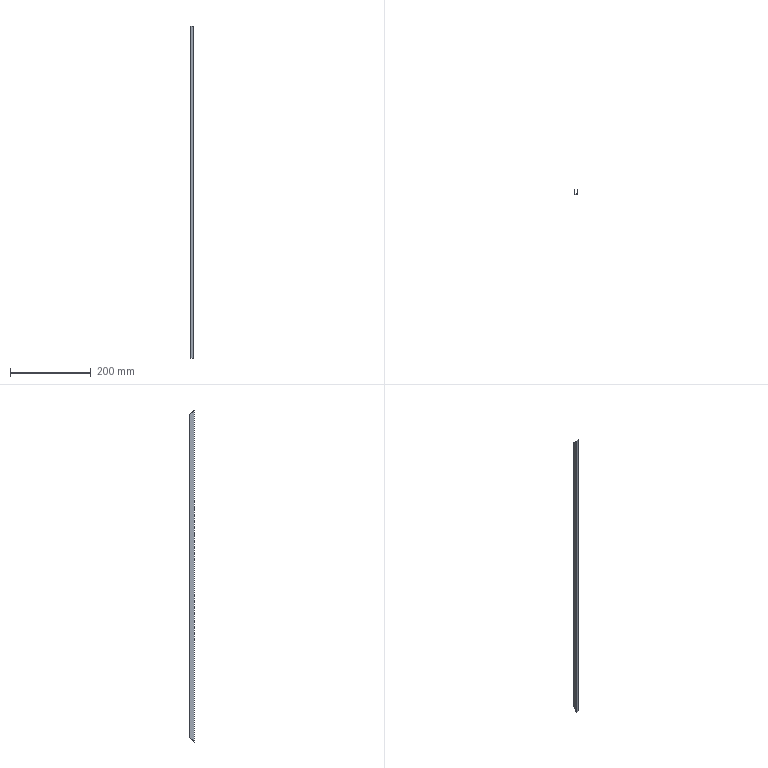Part | STEP file | Friction strip L824 | 1 solid | 10 faces | box 7 x 11 x 824 mm | volume 22001 mm3 | plane 10
STEP:
#1=CARTESIAN_POINT('',(0.,0.,0.));
#2=DIRECTION('',(0.,0.,1.));
#3=DIRECTION('',(1.,0.,0.));
#4=AXIS2_PLACEMENT_3D('',#1,#2,#3);
#5=CARTESIAN_POINT('',(3.5,0.,824.));
#6=VERTEX_POINT('',#5);
#7=CARTESIAN_POINT('',(3.5,0.,0.));
#8=VERTEX_POINT('',#7);
#9=CARTESIAN_POINT('',(3.5,0.,824.));
#10=DIRECTION('',(0.,0.,-1.));
#11=VECTOR('',#10,1.);
#12=LINE('',#9,#11);
#13=CARTESIAN_POINT('',(3.5,0.,824.));
#14=DIRECTION('',(-1.,0.,0.));
#15=DIRECTION('',(0.,-1.,0.));
#16=AXIS2_PLACEMENT_3D('',#13,#14,#15);
#17=PLANE('',#16);
#18=CARTESIAN_POINT('',(0.,0.));
#19=DIRECTION('',(0.,-1.));
#20=VECTOR('',#19,1.);
#21=LINE('',#18,#20);
#22=(GEOMETRIC_REPRESENTATION_CONTEXT(2)PARAMETRIC_REPRESENTATION_CONTEXT()REPRESENTATION_CONTEXT('',''));
#23=DEFINITIONAL_REPRESENTATION('',(#21),#22);
#24=PCURVE('',#17,#23);
#25=CARTESIAN_POINT('',(-3.5,0.,824.));
#26=DIRECTION('',(0.,1.,0.));
#27=DIRECTION('',(0.,0.,1.));
#28=AXIS2_PLACEMENT_3D('',#25,#26,#27);
#29=PLANE('',#28);
#30=CARTESIAN_POINT('',(0.,7.));
#31=DIRECTION('',(-1.,0.));
#32=VECTOR('',#31,1.);
#33=LINE('',#30,#32);
#34=(GEOMETRIC_REPRESENTATION_CONTEXT(2)PARAMETRIC_REPRESENTATION_CONTEXT()REPRESENTATION_CONTEXT('',''));
#35=DEFINITIONAL_REPRESENTATION('',(#33),#34);
#36=PCURVE('',#29,#35);
#37=SURFACE_CURVE('',#12,(#24,#36),.PCURVE_S1.);
#38=EDGE_CURVE('',#6,#8,#37,.T.);
#39=ORIENTED_EDGE('',*,*,#38,.T.);
#40=CARTESIAN_POINT('',(3.5,11.,11.));
#41=VERTEX_POINT('',#40);
#42=CARTESIAN_POINT('',(3.5,0.,0.));
#43=DIRECTION('',(0.,0.7071,0.7071));
#44=VECTOR('',#43,1.);
#45=LINE('',#42,#44);
#46=CARTESIAN_POINT('',(0.,-824.));
#47=DIRECTION('',(-0.7071,0.7071));
#48=VECTOR('',#47,1.);
#49=LINE('',#46,#48);
#50=(GEOMETRIC_REPRESENTATION_CONTEXT(2)PARAMETRIC_REPRESENTATION_CONTEXT()REPRESENTATION_CONTEXT('',''));
#51=DEFINITIONAL_REPRESENTATION('',(#49),#50);
#52=PCURVE('',#17,#51);
#53=CARTESIAN_POINT('',(3.5,0.,0.));
#54=DIRECTION('',(0.,-0.7071,0.7071));
#55=DIRECTION('',(0.,-0.7071,-0.7071));
#56=AXIS2_PLACEMENT_3D('',#53,#54,#55);
#57=PLANE('',#56);
#58=CARTESIAN_POINT('',(0.,0.));
#59=DIRECTION('',(-1.,0.));
#60=VECTOR('',#59,1.);
#61=LINE('',#58,#60);
#62=(GEOMETRIC_REPRESENTATION_CONTEXT(2)PARAMETRIC_REPRESENTATION_CONTEXT()REPRESENTATION_CONTEXT('',''));
#63=DEFINITIONAL_REPRESENTATION('',(#61),#62);
#64=PCURVE('',#57,#63);
#65=SURFACE_CURVE('',#45,(#52,#64),.PCURVE_S1.);
#66=EDGE_CURVE('',#8,#41,#65,.T.);
#67=ORIENTED_EDGE('',*,*,#66,.T.);
#68=CARTESIAN_POINT('',(3.5,11.,813.));
#69=VERTEX_POINT('',#68);
#70=CARTESIAN_POINT('',(3.5,11.,824.));
#71=DIRECTION('',(0.,0.,-1.));
#72=VECTOR('',#71,1.);
#73=LINE('',#70,#72);
#74=CARTESIAN_POINT('',(-11.,0.));
#75=DIRECTION('',(0.,-1.));
#76=VECTOR('',#75,1.);
#77=LINE('',#74,#76);
#78=(GEOMETRIC_REPRESENTATION_CONTEXT(2)PARAMETRIC_REPRESENTATION_CONTEXT()REPRESENTATION_CONTEXT('',''));
#79=DEFINITIONAL_REPRESENTATION('',(#77),#78);
#80=PCURVE('',#17,#79);
#81=CARTESIAN_POINT('',(2.5,11.,824.));
#82=DIRECTION('',(0.,1.,0.));
#83=DIRECTION('',(0.,0.,1.));
#84=AXIS2_PLACEMENT_3D('',#81,#82,#83);
#85=PLANE('',#84);
#86=CARTESIAN_POINT('',(0.,1.));
#87=DIRECTION('',(-1.,0.));
#88=VECTOR('',#87,1.);
#89=LINE('',#86,#88);
#90=(GEOMETRIC_REPRESENTATION_CONTEXT(2)PARAMETRIC_REPRESENTATION_CONTEXT()REPRESENTATION_CONTEXT('',''));
#91=DEFINITIONAL_REPRESENTATION('',(#89),#90);
#92=PCURVE('',#85,#91);
#93=SURFACE_CURVE('',#73,(#80,#92),.PCURVE_S1.);
#94=EDGE_CURVE('',#69,#41,#93,.T.);
#95=ORIENTED_EDGE('',*,*,#94,.F.);
#96=CARTESIAN_POINT('',(3.5,0.,824.));
#97=DIRECTION('',(0.,-0.7071,0.7071));
#98=VECTOR('',#97,1.);
#99=LINE('',#96,#98);
#100=CARTESIAN_POINT('',(0.,0.));
#101=DIRECTION('',(0.7071,0.7071));
#102=VECTOR('',#101,1.);
#103=LINE('',#100,#102);
#104=(GEOMETRIC_REPRESENTATION_CONTEXT(2)PARAMETRIC_REPRESENTATION_CONTEXT()REPRESENTATION_CONTEXT('',''));
#105=DEFINITIONAL_REPRESENTATION('',(#103),#104);
#106=PCURVE('',#17,#105);
#107=CARTESIAN_POINT('',(3.5,0.,824.));
#108=DIRECTION('',(0.,-0.7071,-0.7071));
#109=DIRECTION('',(0.,0.7071,-0.7071));
#110=AXIS2_PLACEMENT_3D('',#107,#108,#109);
#111=PLANE('',#110);
#112=CARTESIAN_POINT('',(0.,0.));
#113=DIRECTION('',(-1.,0.));
#114=VECTOR('',#113,1.);
#115=LINE('',#112,#114);
#116=(GEOMETRIC_REPRESENTATION_CONTEXT(2)PARAMETRIC_REPRESENTATION_CONTEXT()REPRESENTATION_CONTEXT('',''));
#117=DEFINITIONAL_REPRESENTATION('',(#115),#116);
#118=PCURVE('',#111,#117);
#119=SURFACE_CURVE('',#99,(#106,#118),.PCURVE_S1.);
#120=EDGE_CURVE('',#69,#6,#119,.T.);
#121=ORIENTED_EDGE('',*,*,#120,.T.);
#122=EDGE_LOOP('',(#39,#67,#95,#121));
#123=FACE_BOUND('',#122,.T.);
#124=ADVANCED_FACE('',(#123),#17,.F.);
#125=CARTESIAN_POINT('',(2.5,11.,11.));
#126=VERTEX_POINT('',#125);
#127=CARTESIAN_POINT('',(3.5,11.,11.));
#128=DIRECTION('',(-1.,0.,0.));
#129=VECTOR('',#128,1.);
#130=LINE('',#127,#129);
#131=CARTESIAN_POINT('',(-813.,1.));
#132=DIRECTION('',(0.,-1.));
#133=VECTOR('',#132,1.);
#134=LINE('',#131,#133);
#135=(GEOMETRIC_REPRESENTATION_CONTEXT(2)PARAMETRIC_REPRESENTATION_CONTEXT()REPRESENTATION_CONTEXT('',''));
#136=DEFINITIONAL_REPRESENTATION('',(#134),#135);
#137=PCURVE('',#85,#136);
#138=CARTESIAN_POINT('',(-15.556,0.));
#139=DIRECTION('',(0.,-1.));
#140=VECTOR('',#139,1.);
#141=LINE('',#138,#140);
#142=(GEOMETRIC_REPRESENTATION_CONTEXT(2)PARAMETRIC_REPRESENTATION_CONTEXT()REPRESENTATION_CONTEXT('',''));
#143=DEFINITIONAL_REPRESENTATION('',(#141),#142);
#144=PCURVE('',#57,#143);
#145=SURFACE_CURVE('',#130,(#137,#144),.PCURVE_S1.);
#146=EDGE_CURVE('',#41,#126,#145,.T.);
#147=ORIENTED_EDGE('',*,*,#146,.T.);
#148=CARTESIAN_POINT('',(2.5,11.,813.));
#149=VERTEX_POINT('',#148);
#150=CARTESIAN_POINT('',(2.5,11.,824.));
#151=DIRECTION('',(0.,0.,-1.));
#152=VECTOR('',#151,1.);
#153=LINE('',#150,#152);
#154=CARTESIAN_POINT('',(0.,0.));
#155=DIRECTION('',(-1.,0.));
#156=VECTOR('',#155,1.);
#157=LINE('',#154,#156);
#158=(GEOMETRIC_REPRESENTATION_CONTEXT(2)PARAMETRIC_REPRESENTATION_CONTEXT()REPRESENTATION_CONTEXT('',''));
#159=DEFINITIONAL_REPRESENTATION('',(#157),#158);
#160=PCURVE('',#85,#159);
#161=CARTESIAN_POINT('',(2.5,0.,824.));
#162=DIRECTION('',(-1.,0.,0.));
#163=DIRECTION('',(0.,-1.,0.));
#164=AXIS2_PLACEMENT_3D('',#161,#162,#163);
#165=PLANE('',#164);
#166=CARTESIAN_POINT('',(-11.,0.));
#167=DIRECTION('',(0.,-1.));
#168=VECTOR('',#167,1.);
#169=LINE('',#166,#168);
#170=(GEOMETRIC_REPRESENTATION_CONTEXT(2)PARAMETRIC_REPRESENTATION_CONTEXT()REPRESENTATION_CONTEXT('',''));
#171=DEFINITIONAL_REPRESENTATION('',(#169),#170);
#172=PCURVE('',#165,#171);
#173=SURFACE_CURVE('',#153,(#160,#172),.PCURVE_S1.);
#174=EDGE_CURVE('',#149,#126,#173,.T.);
#175=ORIENTED_EDGE('',*,*,#174,.F.);
#176=CARTESIAN_POINT('',(3.5,11.,813.));
#177=DIRECTION('',(-1.,0.,0.));
#178=VECTOR('',#177,1.);
#179=LINE('',#176,#178);
#180=CARTESIAN_POINT('',(-11.,1.));
#181=DIRECTION('',(0.,-1.));
#182=VECTOR('',#181,1.);
#183=LINE('',#180,#182);
#184=(GEOMETRIC_REPRESENTATION_CONTEXT(2)PARAMETRIC_REPRESENTATION_CONTEXT()REPRESENTATION_CONTEXT('',''));
#185=DEFINITIONAL_REPRESENTATION('',(#183),#184);
#186=PCURVE('',#85,#185);
#187=CARTESIAN_POINT('',(15.556,0.));
#188=DIRECTION('',(0.,-1.));
#189=VECTOR('',#188,1.);
#190=LINE('',#187,#189);
#191=(GEOMETRIC_REPRESENTATION_CONTEXT(2)PARAMETRIC_REPRESENTATION_CONTEXT()REPRESENTATION_CONTEXT('',''));
#192=DEFINITIONAL_REPRESENTATION('',(#190),#191);
#193=PCURVE('',#111,#192);
#194=SURFACE_CURVE('',#179,(#186,#193),.PCURVE_S1.);
#195=EDGE_CURVE('',#69,#149,#194,.T.);
#196=ORIENTED_EDGE('',*,*,#195,.F.);
#197=ORIENTED_EDGE('',*,*,#94,.T.);
#198=EDGE_LOOP('',(#147,#175,#196,#197));
#199=FACE_BOUND('',#198,.T.);
#200=ADVANCED_FACE('',(#199),#85,.T.);
#201=CARTESIAN_POINT('',(2.5,1.,1.));
#202=VERTEX_POINT('',#201);
#203=CARTESIAN_POINT('',(2.5,412.,412.));
#204=DIRECTION('',(0.,0.7071,0.7071));
#205=VECTOR('',#204,1.);
#206=LINE('',#203,#205);
#207=CARTESIAN_POINT('',(-412.,-412.));
#208=DIRECTION('',(-0.7071,0.7071));
#209=VECTOR('',#208,1.);
#210=LINE('',#207,#209);
#211=(GEOMETRIC_REPRESENTATION_CONTEXT(2)PARAMETRIC_REPRESENTATION_CONTEXT()REPRESENTATION_CONTEXT('',''));
#212=DEFINITIONAL_REPRESENTATION('',(#210),#211);
#213=PCURVE('',#165,#212);
#214=CARTESIAN_POINT('',(-582.656,-1.));
#215=DIRECTION('',(-1.,0.));
#216=VECTOR('',#215,1.);
#217=LINE('',#214,#216);
#218=(GEOMETRIC_REPRESENTATION_CONTEXT(2)PARAMETRIC_REPRESENTATION_CONTEXT()REPRESENTATION_CONTEXT('',''));
#219=DEFINITIONAL_REPRESENTATION('',(#217),#218);
#220=PCURVE('',#57,#219);
#221=SURFACE_CURVE('',#206,(#213,#220),.PCURVE_S1.);
#222=EDGE_CURVE('',#202,#126,#221,.T.);
#223=ORIENTED_EDGE('',*,*,#222,.F.);
#224=CARTESIAN_POINT('',(2.5,1.,823.));
#225=VERTEX_POINT('',#224);
#226=CARTESIAN_POINT('',(2.5,1.,824.));
#227=DIRECTION('',(0.,0.,-1.));
#228=VECTOR('',#227,1.);
#229=LINE('',#226,#228);
#230=CARTESIAN_POINT('',(-1.,0.));
#231=DIRECTION('',(0.,-1.));
#232=VECTOR('',#231,1.);
#233=LINE('',#230,#232);
#234=(GEOMETRIC_REPRESENTATION_CONTEXT(2)PARAMETRIC_REPRESENTATION_CONTEXT()REPRESENTATION_CONTEXT('',''));
#235=DEFINITIONAL_REPRESENTATION('',(#233),#234);
#236=PCURVE('',#165,#235);
#237=CARTESIAN_POINT('',(-3.5,1.,824.));
#238=DIRECTION('',(0.,1.,0.));
#239=DIRECTION('',(0.,0.,1.));
#240=AXIS2_PLACEMENT_3D('',#237,#238,#239);
#241=PLANE('',#240);
#242=CARTESIAN_POINT('',(0.,6.));
#243=DIRECTION('',(-1.,0.));
#244=VECTOR('',#243,1.);
#245=LINE('',#242,#244);
#246=(GEOMETRIC_REPRESENTATION_CONTEXT(2)PARAMETRIC_REPRESENTATION_CONTEXT()REPRESENTATION_CONTEXT('',''));
#247=DEFINITIONAL_REPRESENTATION('',(#245),#246);
#248=PCURVE('',#241,#247);
#249=SURFACE_CURVE('',#229,(#236,#248),.PCURVE_S1.);
#250=EDGE_CURVE('',#225,#202,#249,.T.);
#251=ORIENTED_EDGE('',*,*,#250,.F.);
#252=CARTESIAN_POINT('',(2.5,0.,824.));
#253=DIRECTION('',(0.,-0.7071,0.7071));
#254=VECTOR('',#253,1.);
#255=LINE('',#252,#254);
#256=CARTESIAN_POINT('',(0.,0.));
#257=DIRECTION('',(0.7071,0.7071));
#258=VECTOR('',#257,1.);
#259=LINE('',#256,#258);
#260=(GEOMETRIC_REPRESENTATION_CONTEXT(2)PARAMETRIC_REPRESENTATION_CONTEXT()REPRESENTATION_CONTEXT('',''));
#261=DEFINITIONAL_REPRESENTATION('',(#259),#260);
#262=PCURVE('',#165,#261);
#263=CARTESIAN_POINT('',(0.,-1.));
#264=DIRECTION('',(-1.,0.));
#265=VECTOR('',#264,1.);
#266=LINE('',#263,#265);
#267=(GEOMETRIC_REPRESENTATION_CONTEXT(2)PARAMETRIC_REPRESENTATION_CONTEXT()REPRESENTATION_CONTEXT('',''));
#268=DEFINITIONAL_REPRESENTATION('',(#266),#267);
#269=PCURVE('',#111,#268);
#270=SURFACE_CURVE('',#255,(#262,#269),.PCURVE_S1.);
#271=EDGE_CURVE('',#149,#225,#270,.T.);
#272=ORIENTED_EDGE('',*,*,#271,.F.);
#273=ORIENTED_EDGE('',*,*,#174,.T.);
#274=EDGE_LOOP('',(#223,#251,#272,#273));
#275=FACE_BOUND('',#274,.T.);
#276=ADVANCED_FACE('',(#275),#165,.T.);
#277=CARTESIAN_POINT('',(-2.5,1.,1.));
#278=VERTEX_POINT('',#277);
#279=CARTESIAN_POINT('',(-3.5,1.,1.));
#280=DIRECTION('',(1.,0.,0.));
#281=VECTOR('',#280,1.);
#282=LINE('',#279,#281);
#283=CARTESIAN_POINT('',(-823.,0.));
#284=DIRECTION('',(0.,1.));
#285=VECTOR('',#284,1.);
#286=LINE('',#283,#285);
#287=(GEOMETRIC_REPRESENTATION_CONTEXT(2)PARAMETRIC_REPRESENTATION_CONTEXT()REPRESENTATION_CONTEXT('',''));
#288=DEFINITIONAL_REPRESENTATION('',(#286),#287);
#289=PCURVE('',#241,#288);
#290=CARTESIAN_POINT('',(-1.414,-7.));
#291=DIRECTION('',(0.,1.));
#292=VECTOR('',#291,1.);
#293=LINE('',#290,#292);
#294=(GEOMETRIC_REPRESENTATION_CONTEXT(2)PARAMETRIC_REPRESENTATION_CONTEXT()REPRESENTATION_CONTEXT('',''));
#295=DEFINITIONAL_REPRESENTATION('',(#293),#294);
#296=PCURVE('',#57,#295);
#297=SURFACE_CURVE('',#282,(#289,#296),.PCURVE_S1.);
#298=EDGE_CURVE('',#278,#202,#297,.T.);
#299=ORIENTED_EDGE('',*,*,#298,.F.);
#300=CARTESIAN_POINT('',(-2.5,1.,823.));
#301=VERTEX_POINT('',#300);
#302=CARTESIAN_POINT('',(-2.5,1.,824.));
#303=DIRECTION('',(0.,0.,-1.));
#304=VECTOR('',#303,1.);
#305=LINE('',#302,#304);
#306=CARTESIAN_POINT('',(0.,1.));
#307=DIRECTION('',(-1.,0.));
#308=VECTOR('',#307,1.);
#309=LINE('',#306,#308);
#310=(GEOMETRIC_REPRESENTATION_CONTEXT(2)PARAMETRIC_REPRESENTATION_CONTEXT()REPRESENTATION_CONTEXT('',''));
#311=DEFINITIONAL_REPRESENTATION('',(#309),#310);
#312=PCURVE('',#241,#311);
#313=CARTESIAN_POINT('',(-2.5,11.,824.));
#314=DIRECTION('',(1.,0.,0.));
#315=DIRECTION('',(0.,1.,0.));
#316=AXIS2_PLACEMENT_3D('',#313,#314,#315);
#317=PLANE('',#316);
#318=CARTESIAN_POINT('',(-10.,0.));
#319=DIRECTION('',(0.,-1.));
#320=VECTOR('',#319,1.);
#321=LINE('',#318,#320);
#322=(GEOMETRIC_REPRESENTATION_CONTEXT(2)PARAMETRIC_REPRESENTATION_CONTEXT()REPRESENTATION_CONTEXT('',''));
#323=DEFINITIONAL_REPRESENTATION('',(#321),#322);
#324=PCURVE('',#317,#323);
#325=SURFACE_CURVE('',#305,(#312,#324),.PCURVE_S1.);
#326=EDGE_CURVE('',#301,#278,#325,.T.);
#327=ORIENTED_EDGE('',*,*,#326,.F.);
#328=CARTESIAN_POINT('',(-3.5,1.,823.));
#329=DIRECTION('',(-1.,0.,0.));
#330=VECTOR('',#329,1.);
#331=LINE('',#328,#330);
#332=CARTESIAN_POINT('',(-1.,0.));
#333=DIRECTION('',(0.,-1.));
#334=VECTOR('',#333,1.);
#335=LINE('',#332,#334);
#336=(GEOMETRIC_REPRESENTATION_CONTEXT(2)PARAMETRIC_REPRESENTATION_CONTEXT()REPRESENTATION_CONTEXT('',''));
#337=DEFINITIONAL_REPRESENTATION('',(#335),#336);
#338=PCURVE('',#241,#337);
#339=CARTESIAN_POINT('',(1.414,-7.));
#340=DIRECTION('',(0.,-1.));
#341=VECTOR('',#340,1.);
#342=LINE('',#339,#341);
#343=(GEOMETRIC_REPRESENTATION_CONTEXT(2)PARAMETRIC_REPRESENTATION_CONTEXT()REPRESENTATION_CONTEXT('',''));
#344=DEFINITIONAL_REPRESENTATION('',(#342),#343);
#345=PCURVE('',#111,#344);
#346=SURFACE_CURVE('',#331,(#338,#345),.PCURVE_S1.);
#347=EDGE_CURVE('',#225,#301,#346,.T.);
#348=ORIENTED_EDGE('',*,*,#347,.F.);
#349=ORIENTED_EDGE('',*,*,#250,.T.);
#350=EDGE_LOOP('',(#299,#327,#348,#349));
#351=FACE_BOUND('',#350,.T.);
#352=ADVANCED_FACE('',(#351),#241,.T.);
#353=CARTESIAN_POINT('',(-2.5,11.,11.));
#354=VERTEX_POINT('',#353);
#355=CARTESIAN_POINT('',(-2.5,417.5,417.5));
#356=DIRECTION('',(0.,-0.7071,-0.7071));
#357=VECTOR('',#356,1.);
#358=LINE('',#355,#357);
#359=CARTESIAN_POINT('',(406.5,-406.5));
#360=DIRECTION('',(-0.7071,-0.7071));
#361=VECTOR('',#360,1.);
#362=LINE('',#359,#361);
#363=(GEOMETRIC_REPRESENTATION_CONTEXT(2)PARAMETRIC_REPRESENTATION_CONTEXT()REPRESENTATION_CONTEXT('',''));
#364=DEFINITIONAL_REPRESENTATION('',(#362),#363);
#365=PCURVE('',#317,#364);
#366=CARTESIAN_POINT('',(-590.434,-6.));
#367=DIRECTION('',(1.,0.));
#368=VECTOR('',#367,1.);
#369=LINE('',#366,#368);
#370=(GEOMETRIC_REPRESENTATION_CONTEXT(2)PARAMETRIC_REPRESENTATION_CONTEXT()REPRESENTATION_CONTEXT('',''));
#371=DEFINITIONAL_REPRESENTATION('',(#369),#370);
#372=PCURVE('',#57,#371);
#373=SURFACE_CURVE('',#358,(#365,#372),.PCURVE_S1.);
#374=EDGE_CURVE('',#354,#278,#373,.T.);
#375=ORIENTED_EDGE('',*,*,#374,.F.);
#376=CARTESIAN_POINT('',(-2.5,11.,813.));
#377=VERTEX_POINT('',#376);
#378=CARTESIAN_POINT('',(-2.5,11.,824.));
#379=DIRECTION('',(0.,0.,-1.));
#380=VECTOR('',#379,1.);
#381=LINE('',#378,#380);
#382=CARTESIAN_POINT('',(0.,0.));
#383=DIRECTION('',(0.,-1.));
#384=VECTOR('',#383,1.);
#385=LINE('',#382,#384);
#386=(GEOMETRIC_REPRESENTATION_CONTEXT(2)PARAMETRIC_REPRESENTATION_CONTEXT()REPRESENTATION_CONTEXT('',''));
#387=DEFINITIONAL_REPRESENTATION('',(#385),#386);
#388=PCURVE('',#317,#387);
#389=CARTESIAN_POINT('',(-3.5,11.,824.));
#390=DIRECTION('',(0.,1.,0.));
#391=DIRECTION('',(0.,0.,1.));
#392=AXIS2_PLACEMENT_3D('',#389,#390,#391);
#393=PLANE('',#392);
#394=CARTESIAN_POINT('',(0.,1.));
#395=DIRECTION('',(-1.,0.));
#396=VECTOR('',#395,1.);
#397=LINE('',#394,#396);
#398=(GEOMETRIC_REPRESENTATION_CONTEXT(2)PARAMETRIC_REPRESENTATION_CONTEXT()REPRESENTATION_CONTEXT('',''));
#399=DEFINITIONAL_REPRESENTATION('',(#397),#398);
#400=PCURVE('',#393,#399);
#401=SURFACE_CURVE('',#381,(#388,#400),.PCURVE_S1.);
#402=EDGE_CURVE('',#377,#354,#401,.T.);
#403=ORIENTED_EDGE('',*,*,#402,.F.);
#404=CARTESIAN_POINT('',(-2.5,5.5,818.5));
#405=DIRECTION('',(0.,0.7071,-0.7071));
#406=VECTOR('',#405,1.);
#407=LINE('',#404,#406);
#408=CARTESIAN_POINT('',(-5.5,-5.5));
#409=DIRECTION('',(0.7071,-0.7071));
#410=VECTOR('',#409,1.);
#411=LINE('',#408,#410);
#412=(GEOMETRIC_REPRESENTATION_CONTEXT(2)PARAMETRIC_REPRESENTATION_CONTEXT()REPRESENTATION_CONTEXT('',''));
#413=DEFINITIONAL_REPRESENTATION('',(#411),#412);
#414=PCURVE('',#317,#413);
#415=CARTESIAN_POINT('',(7.778,-6.));
#416=DIRECTION('',(1.,0.));
#417=VECTOR('',#416,1.);
#418=LINE('',#415,#417);
#419=(GEOMETRIC_REPRESENTATION_CONTEXT(2)PARAMETRIC_REPRESENTATION_CONTEXT()REPRESENTATION_CONTEXT('',''));
#420=DEFINITIONAL_REPRESENTATION('',(#418),#419);
#421=PCURVE('',#111,#420);
#422=SURFACE_CURVE('',#407,(#414,#421),.PCURVE_S1.);
#423=EDGE_CURVE('',#301,#377,#422,.T.);
#424=ORIENTED_EDGE('',*,*,#423,.F.);
#425=ORIENTED_EDGE('',*,*,#326,.T.);
#426=EDGE_LOOP('',(#375,#403,#424,#425));
#427=FACE_BOUND('',#426,.T.);
#428=ADVANCED_FACE('',(#427),#317,.T.);
#429=CARTESIAN_POINT('',(-3.5,11.,11.));
#430=VERTEX_POINT('',#429);
#431=CARTESIAN_POINT('',(3.5,11.,11.));
#432=DIRECTION('',(-1.,0.,0.));
#433=VECTOR('',#432,1.);
#434=LINE('',#431,#433);
#435=CARTESIAN_POINT('',(-813.,7.));
#436=DIRECTION('',(0.,-1.));
#437=VECTOR('',#436,1.);
#438=LINE('',#435,#437);
#439=(GEOMETRIC_REPRESENTATION_CONTEXT(2)PARAMETRIC_REPRESENTATION_CONTEXT()REPRESENTATION_CONTEXT('',''));
#440=DEFINITIONAL_REPRESENTATION('',(#438),#439);
#441=PCURVE('',#393,#440);
#442=CARTESIAN_POINT('',(-15.556,0.));
#443=DIRECTION('',(0.,-1.));
#444=VECTOR('',#443,1.);
#445=LINE('',#442,#444);
#446=(GEOMETRIC_REPRESENTATION_CONTEXT(2)PARAMETRIC_REPRESENTATION_CONTEXT()REPRESENTATION_CONTEXT('',''));
#447=DEFINITIONAL_REPRESENTATION('',(#445),#446);
#448=PCURVE('',#57,#447);
#449=SURFACE_CURVE('',#434,(#441,#448),.PCURVE_S1.);
#450=EDGE_CURVE('',#354,#430,#449,.T.);
#451=ORIENTED_EDGE('',*,*,#450,.T.);
#452=CARTESIAN_POINT('',(-3.5,11.,813.));
#453=VERTEX_POINT('',#452);
#454=CARTESIAN_POINT('',(-3.5,11.,824.));
#455=DIRECTION('',(0.,0.,-1.));
#456=VECTOR('',#455,1.);
#457=LINE('',#454,#456);
#458=CARTESIAN_POINT('',(0.,0.));
#459=DIRECTION('',(-1.,0.));
#460=VECTOR('',#459,1.);
#461=LINE('',#458,#460);
#462=(GEOMETRIC_REPRESENTATION_CONTEXT(2)PARAMETRIC_REPRESENTATION_CONTEXT()REPRESENTATION_CONTEXT('',''));
#463=DEFINITIONAL_REPRESENTATION('',(#461),#462);
#464=PCURVE('',#393,#463);
#465=CARTESIAN_POINT('',(-3.5,11.,824.));
#466=DIRECTION('',(1.,0.,0.));
#467=DIRECTION('',(0.,1.,0.));
#468=AXIS2_PLACEMENT_3D('',#465,#466,#467);
#469=PLANE('',#468);
#470=CARTESIAN_POINT('',(0.,0.));
#471=DIRECTION('',(0.,-1.));
#472=VECTOR('',#471,1.);
#473=LINE('',#470,#472);
#474=(GEOMETRIC_REPRESENTATION_CONTEXT(2)PARAMETRIC_REPRESENTATION_CONTEXT()REPRESENTATION_CONTEXT('',''));
#475=DEFINITIONAL_REPRESENTATION('',(#473),#474);
#476=PCURVE('',#469,#475);
#477=SURFACE_CURVE('',#457,(#464,#476),.PCURVE_S1.);
#478=EDGE_CURVE('',#453,#430,#477,.T.);
#479=ORIENTED_EDGE('',*,*,#478,.F.);
#480=CARTESIAN_POINT('',(3.5,11.,813.));
#481=DIRECTION('',(-1.,0.,0.));
#482=VECTOR('',#481,1.);
#483=LINE('',#480,#482);
#484=CARTESIAN_POINT('',(-11.,7.));
#485=DIRECTION('',(0.,-1.));
#486=VECTOR('',#485,1.);
#487=LINE('',#484,#486);
#488=(GEOMETRIC_REPRESENTATION_CONTEXT(2)PARAMETRIC_REPRESENTATION_CONTEXT()REPRESENTATION_CONTEXT('',''));
#489=DEFINITIONAL_REPRESENTATION('',(#487),#488);
#490=PCURVE('',#393,#489);
#491=CARTESIAN_POINT('',(15.556,0.));
#492=DIRECTION('',(0.,-1.));
#493=VECTOR('',#492,1.);
#494=LINE('',#491,#493);
#495=(GEOMETRIC_REPRESENTATION_CONTEXT(2)PARAMETRIC_REPRESENTATION_CONTEXT()REPRESENTATION_CONTEXT('',''));
#496=DEFINITIONAL_REPRESENTATION('',(#494),#495);
#497=PCURVE('',#111,#496);
#498=SURFACE_CURVE('',#483,(#490,#497),.PCURVE_S1.);
#499=EDGE_CURVE('',#377,#453,#498,.T.);
#500=ORIENTED_EDGE('',*,*,#499,.F.);
#501=ORIENTED_EDGE('',*,*,#402,.T.);
#502=EDGE_LOOP('',(#451,#479,#500,#501));
#503=FACE_BOUND('',#502,.T.);
#504=ADVANCED_FACE('',(#503),#393,.T.);
#505=ORIENTED_EDGE('',*,*,#478,.T.);
#506=CARTESIAN_POINT('',(-3.5,0.,0.));
#507=VERTEX_POINT('',#506);
#508=CARTESIAN_POINT('',(-3.5,0.,0.));
#509=DIRECTION('',(0.,0.7071,0.7071));
#510=VECTOR('',#509,1.);
#511=LINE('',#508,#510);
#512=CARTESIAN_POINT('',(-11.,-824.));
#513=DIRECTION('',(0.7071,0.7071));
#514=VECTOR('',#513,1.);
#515=LINE('',#512,#514);
#516=(GEOMETRIC_REPRESENTATION_CONTEXT(2)PARAMETRIC_REPRESENTATION_CONTEXT()REPRESENTATION_CONTEXT('',''));
#517=DEFINITIONAL_REPRESENTATION('',(#515),#516);
#518=PCURVE('',#469,#517);
#519=CARTESIAN_POINT('',(0.,-7.));
#520=DIRECTION('',(-1.,0.));
#521=VECTOR('',#520,1.);
#522=LINE('',#519,#521);
#523=(GEOMETRIC_REPRESENTATION_CONTEXT(2)PARAMETRIC_REPRESENTATION_CONTEXT()REPRESENTATION_CONTEXT('',''));
#524=DEFINITIONAL_REPRESENTATION('',(#522),#523);
#525=PCURVE('',#57,#524);
#526=SURFACE_CURVE('',#511,(#518,#525),.PCURVE_S1.);
#527=EDGE_CURVE('',#507,#430,#526,.T.);
#528=ORIENTED_EDGE('',*,*,#527,.F.);
#529=CARTESIAN_POINT('',(-3.5,0.,824.));
#530=VERTEX_POINT('',#529);
#531=CARTESIAN_POINT('',(-3.5,0.,824.));
#532=DIRECTION('',(0.,0.,-1.));
#533=VECTOR('',#532,1.);
#534=LINE('',#531,#533);
#535=CARTESIAN_POINT('',(-11.,0.));
#536=DIRECTION('',(0.,-1.));
#537=VECTOR('',#536,1.);
#538=LINE('',#535,#537);
#539=(GEOMETRIC_REPRESENTATION_CONTEXT(2)PARAMETRIC_REPRESENTATION_CONTEXT()REPRESENTATION_CONTEXT('',''));
#540=DEFINITIONAL_REPRESENTATION('',(#538),#539);
#541=PCURVE('',#469,#540);
#542=CARTESIAN_POINT('',(0.,0.));
#543=DIRECTION('',(-1.,0.));
#544=VECTOR('',#543,1.);
#545=LINE('',#542,#544);
#546=(GEOMETRIC_REPRESENTATION_CONTEXT(2)PARAMETRIC_REPRESENTATION_CONTEXT()REPRESENTATION_CONTEXT('',''));
#547=DEFINITIONAL_REPRESENTATION('',(#545),#546);
#548=PCURVE('',#29,#547);
#549=SURFACE_CURVE('',#534,(#541,#548),.PCURVE_S1.);
#550=EDGE_CURVE('',#530,#507,#549,.T.);
#551=ORIENTED_EDGE('',*,*,#550,.F.);
#552=CARTESIAN_POINT('',(-3.5,0.,824.));
#553=DIRECTION('',(0.,-0.7071,0.7071));
#554=VECTOR('',#553,1.);
#555=LINE('',#552,#554);
#556=CARTESIAN_POINT('',(-11.,0.));
#557=DIRECTION('',(-0.7071,0.7071));
#558=VECTOR('',#557,1.);
#559=LINE('',#556,#558);
#560=(GEOMETRIC_REPRESENTATION_CONTEXT(2)PARAMETRIC_REPRESENTATION_CONTEXT()REPRESENTATION_CONTEXT('',''));
#561=DEFINITIONAL_REPRESENTATION('',(#559),#560);
#562=PCURVE('',#469,#561);
#563=CARTESIAN_POINT('',(0.,-7.));
#564=DIRECTION('',(-1.,0.));
#565=VECTOR('',#564,1.);
#566=LINE('',#563,#565);
#567=(GEOMETRIC_REPRESENTATION_CONTEXT(2)PARAMETRIC_REPRESENTATION_CONTEXT()REPRESENTATION_CONTEXT('',''));
#568=DEFINITIONAL_REPRESENTATION('',(#566),#567);
#569=PCURVE('',#111,#568);
#570=SURFACE_CURVE('',#555,(#562,#569),.PCURVE_S1.);
#571=EDGE_CURVE('',#453,#530,#570,.T.);
#572=ORIENTED_EDGE('',*,*,#571,.F.);
#573=EDGE_LOOP('',(#505,#528,#551,#572));
#574=FACE_BOUND('',#573,.T.);
#575=ADVANCED_FACE('',(#574),#469,.F.);
#576=CARTESIAN_POINT('',(-3.5,0.,0.));
#577=DIRECTION('',(1.,0.,0.));
#578=VECTOR('',#577,1.);
#579=LINE('',#576,#578);
#580=CARTESIAN_POINT('',(-824.,0.));
#581=DIRECTION('',(0.,1.));
#582=VECTOR('',#581,1.);
#583=LINE('',#580,#582);
#584=(GEOMETRIC_REPRESENTATION_CONTEXT(2)PARAMETRIC_REPRESENTATION_CONTEXT()REPRESENTATION_CONTEXT('',''));
#585=DEFINITIONAL_REPRESENTATION('',(#583),#584);
#586=PCURVE('',#29,#585);
#587=CARTESIAN_POINT('',(0.,-7.));
#588=DIRECTION('',(0.,1.));
#589=VECTOR('',#588,1.);
#590=LINE('',#587,#589);
#591=(GEOMETRIC_REPRESENTATION_CONTEXT(2)PARAMETRIC_REPRESENTATION_CONTEXT()REPRESENTATION_CONTEXT('',''));
#592=DEFINITIONAL_REPRESENTATION('',(#590),#591);
#593=PCURVE('',#57,#592);
#594=SURFACE_CURVE('',#579,(#586,#593),.PCURVE_S1.);
#595=EDGE_CURVE('',#507,#8,#594,.T.);
#596=ORIENTED_EDGE('',*,*,#595,.T.);
#597=ORIENTED_EDGE('',*,*,#38,.F.);
#598=CARTESIAN_POINT('',(-3.5,0.,824.));
#599=DIRECTION('',(1.,0.,0.));
#600=VECTOR('',#599,1.);
#601=LINE('',#598,#600);
#602=CARTESIAN_POINT('',(0.,0.));
#603=DIRECTION('',(0.,1.));
#604=VECTOR('',#603,1.);
#605=LINE('',#602,#604);
#606=(GEOMETRIC_REPRESENTATION_CONTEXT(2)PARAMETRIC_REPRESENTATION_CONTEXT()REPRESENTATION_CONTEXT('',''));
#607=DEFINITIONAL_REPRESENTATION('',(#605),#606);
#608=PCURVE('',#29,#607);
#609=CARTESIAN_POINT('',(0.,-7.));
#610=DIRECTION('',(0.,1.));
#611=VECTOR('',#610,1.);
#612=LINE('',#609,#611);
#613=(GEOMETRIC_REPRESENTATION_CONTEXT(2)PARAMETRIC_REPRESENTATION_CONTEXT()REPRESENTATION_CONTEXT('',''));
#614=DEFINITIONAL_REPRESENTATION('',(#612),#613);
#615=PCURVE('',#111,#614);
#616=SURFACE_CURVE('',#601,(#608,#615),.PCURVE_S1.);
#617=EDGE_CURVE('',#530,#6,#616,.T.);
#618=ORIENTED_EDGE('',*,*,#617,.F.);
#619=ORIENTED_EDGE('',*,*,#550,.T.);
#620=EDGE_LOOP('',(#596,#597,#618,#619));
#621=FACE_BOUND('',#620,.T.);
#622=ADVANCED_FACE('',(#621),#29,.F.);
#623=ORIENTED_EDGE('',*,*,#271,.T.);
#624=ORIENTED_EDGE('',*,*,#347,.T.);
#625=ORIENTED_EDGE('',*,*,#423,.T.);
#626=ORIENTED_EDGE('',*,*,#499,.T.);
#627=ORIENTED_EDGE('',*,*,#571,.T.);
#628=ORIENTED_EDGE('',*,*,#617,.T.);
#629=ORIENTED_EDGE('',*,*,#120,.F.);
#630=ORIENTED_EDGE('',*,*,#195,.T.);
#631=EDGE_LOOP('',(#623,#624,#625,#626,#627,#628,#629,#630));
#632=FACE_BOUND('',#631,.T.);
#633=ADVANCED_FACE('',(#632),#111,.F.);
#634=ORIENTED_EDGE('',*,*,#222,.T.);
#635=ORIENTED_EDGE('',*,*,#146,.F.);
#636=ORIENTED_EDGE('',*,*,#66,.F.);
#637=ORIENTED_EDGE('',*,*,#595,.F.);
#638=ORIENTED_EDGE('',*,*,#527,.T.);
#639=ORIENTED_EDGE('',*,*,#450,.F.);
#640=ORIENTED_EDGE('',*,*,#374,.T.);
#641=ORIENTED_EDGE('',*,*,#298,.T.);
#642=EDGE_LOOP('',(#634,#635,#636,#637,#638,#639,#640,#641));
#643=FACE_BOUND('',#642,.T.);
#644=ADVANCED_FACE('',(#643),#57,.F.);
#645=CLOSED_SHELL('',(#124,#200,#276,#352,#428,#504,#575,#622,#633,#644));
#646=MANIFOLD_SOLID_BREP('',#645);
#647=(LENGTH_UNIT()NAMED_UNIT(*)SI_UNIT(.MILLI.,.METRE.));
#648=UNCERTAINTY_MEASURE_WITH_UNIT(LENGTH_MEASURE(0.0000001),#647,'','');
#649=(NAMED_UNIT(*)PLANE_ANGLE_UNIT()SI_UNIT($,.RADIAN.));
#650=(NAMED_UNIT(*)SI_UNIT($,.STERADIAN.)SOLID_ANGLE_UNIT());
#651=(GEOMETRIC_REPRESENTATION_CONTEXT(3)GLOBAL_UNCERTAINTY_ASSIGNED_CONTEXT((#648))GLOBAL_UNIT_ASSIGNED_CONTEXT((#647,#649,#650))REPRESENTATION_CONTEXT('',''));
#652=ADVANCED_BREP_SHAPE_REPRESENTATION('',(#4,#646),#651);